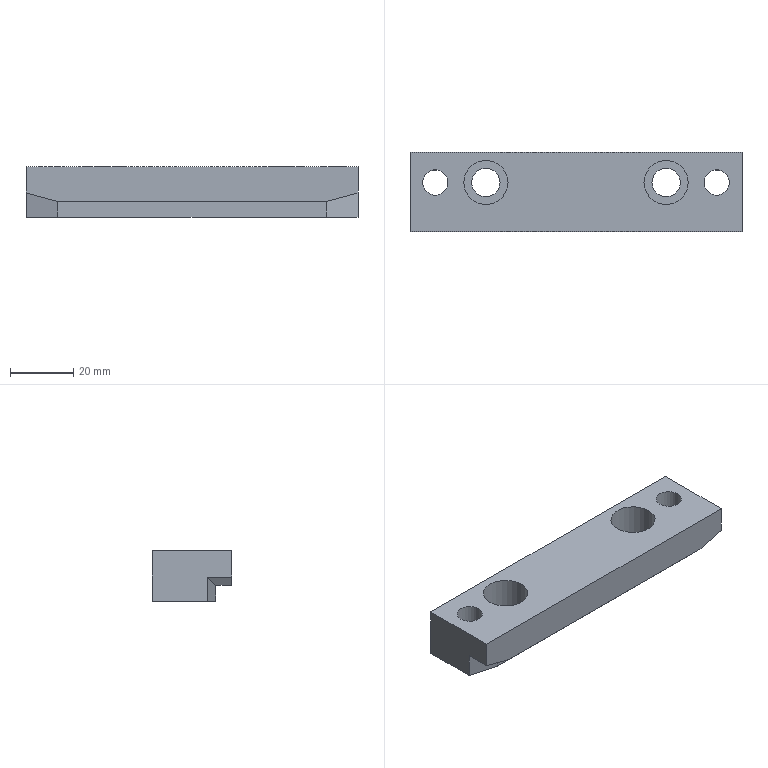Part | STEP file | 1 solid | 20 faces | box 105 x 25 x 16 mm | volume 33608 mm3 | plane 14 | cylinder 6 | commonest cylinder face diameters 8 x2 9 x2 14 x2
STEP:
#1=CARTESIAN_POINT('',(20.,96.9,3.));
#2=VERTEX_POINT('',#1);
#3=CARTESIAN_POINT('',(30.,99.58,5.679));
#4=VERTEX_POINT('',#3);
#5=CARTESIAN_POINT('',(35.23,100.981,7.081));
#6=DIRECTION('',(0.9351,0.2506,0.2506));
#7=VECTOR('',#6,1.);
#8=LINE('',#5,#7);
#9=EDGE_CURVE('',#2,#4,#8,.T.);
#10=ORIENTED_EDGE('',*,*,#9,.T.);
#11=CARTESIAN_POINT('',(30.,91.9,5.679));
#12=VERTEX_POINT('',#11);
#13=CARTESIAN_POINT('',(30.,89.4,5.679));
#14=DIRECTION('',(0.,-1.,0.));
#15=VECTOR('',#14,1.);
#16=LINE('',#13,#15);
#17=EDGE_CURVE('',#4,#12,#16,.T.);
#18=ORIENTED_EDGE('',*,*,#17,.T.);
#19=CARTESIAN_POINT('',(20.,91.9,3.));
#20=VERTEX_POINT('',#19);
#21=CARTESIAN_POINT('',(27.33,91.9,4.964));
#22=DIRECTION('',(-0.9659,0.,-0.2588));
#23=VECTOR('',#22,1.);
#24=LINE('',#21,#23);
#25=EDGE_CURVE('',#12,#20,#24,.T.);
#26=ORIENTED_EDGE('',*,*,#25,.T.);
#27=CARTESIAN_POINT('',(20.,97.08,3.));
#28=DIRECTION('',(0.,1.,0.));
#29=VECTOR('',#28,1.);
#30=LINE('',#27,#29);
#31=EDGE_CURVE('',#20,#2,#30,.T.);
#32=ORIENTED_EDGE('',*,*,#31,.T.);
#33=EDGE_LOOP('',(#10,#18,#26,#32));
#34=FACE_OUTER_BOUND('',#33,.T.);
#35=CARTESIAN_POINT('',(30.,119.4,5.679));
#36=DIRECTION('',(0.2588,0.,-0.9659));
#37=DIRECTION('',(0.9659,0.,0.2588));
#38=AXIS2_PLACEMENT_3D('',#35,#36,#37);
#39=PLANE('',#38);
#40=ADVANCED_FACE('',(#34),#39,.T.);
#41=CARTESIAN_POINT('',(-65.,96.9,3.));
#42=VERTEX_POINT('',#41);
#43=CARTESIAN_POINT('',(-125.,96.9,3.));
#44=DIRECTION('',(-1.,0.,0.));
#45=VECTOR('',#44,1.);
#46=LINE('',#43,#45);
#47=EDGE_CURVE('',#2,#42,#46,.T.);
#48=ORIENTED_EDGE('',*,*,#47,.F.);
#49=ORIENTED_EDGE('',*,*,#31,.F.);
#50=CARTESIAN_POINT('',(-65.,91.9,3.));
#51=VERTEX_POINT('',#50);
#52=CARTESIAN_POINT('',(-35.,91.9,3.));
#53=DIRECTION('',(1.,0.,0.));
#54=VECTOR('',#53,1.);
#55=LINE('',#52,#54);
#56=EDGE_CURVE('',#51,#20,#55,.T.);
#57=ORIENTED_EDGE('',*,*,#56,.F.);
#58=CARTESIAN_POINT('',(-65.,97.08,3.));
#59=DIRECTION('',(0.,1.,0.));
#60=VECTOR('',#59,1.);
#61=LINE('',#58,#60);
#62=EDGE_CURVE('',#51,#42,#61,.T.);
#63=ORIENTED_EDGE('',*,*,#62,.T.);
#64=EDGE_LOOP('',(#48,#49,#57,#63));
#65=FACE_OUTER_BOUND('',#64,.T.);
#66=CARTESIAN_POINT('',(-46.,107.4,3.));
#67=DIRECTION('',(0.,0.,1.));
#68=DIRECTION('',(-1.,0.,0.));
#69=AXIS2_PLACEMENT_3D('',#66,#67,#68);
#70=PLANE('',#69);
#71=ADVANCED_FACE('',(#65),#70,.F.);
#72=CARTESIAN_POINT('',(-75.,99.58,5.679));
#73=VERTEX_POINT('',#72);
#74=CARTESIAN_POINT('',(-80.23,100.981,7.081));
#75=DIRECTION('',(-0.9351,0.2506,0.2506));
#76=VECTOR('',#75,1.);
#77=LINE('',#74,#76);
#78=EDGE_CURVE('',#42,#73,#77,.T.);
#79=ORIENTED_EDGE('',*,*,#78,.F.);
#80=ORIENTED_EDGE('',*,*,#62,.F.);
#81=CARTESIAN_POINT('',(-75.,91.9,5.679));
#82=VERTEX_POINT('',#81);
#83=CARTESIAN_POINT('',(-72.33,91.9,4.964));
#84=DIRECTION('',(0.9659,0.,-0.2588));
#85=VECTOR('',#84,1.);
#86=LINE('',#83,#85);
#87=EDGE_CURVE('',#82,#51,#86,.T.);
#88=ORIENTED_EDGE('',*,*,#87,.F.);
#89=CARTESIAN_POINT('',(-75.,89.4,5.679));
#90=DIRECTION('',(0.,-1.,0.));
#91=VECTOR('',#90,1.);
#92=LINE('',#89,#91);
#93=EDGE_CURVE('',#73,#82,#92,.T.);
#94=ORIENTED_EDGE('',*,*,#93,.F.);
#95=EDGE_LOOP('',(#79,#80,#88,#94));
#96=FACE_OUTER_BOUND('',#95,.T.);
#97=CARTESIAN_POINT('',(-75.,119.4,5.679));
#98=DIRECTION('',(-0.2588,0.,-0.9659));
#99=DIRECTION('',(-0.9659,0.,0.2588));
#100=AXIS2_PLACEMENT_3D('',#97,#98,#99);
#101=PLANE('',#100);
#102=ADVANCED_FACE('',(#96),#101,.T.);
#103=CARTESIAN_POINT('',(-64.998,96.9,-2.));
#104=VERTEX_POINT('',#103);
#105=CARTESIAN_POINT('',(-64.998,96.9,14.));
#106=DIRECTION('',(0.,0.,1.));
#107=VECTOR('',#106,1.);
#108=LINE('',#105,#107);
#109=EDGE_CURVE('',#104,#42,#108,.T.);
#110=ORIENTED_EDGE('',*,*,#109,.T.);
#111=ORIENTED_EDGE('',*,*,#78,.T.);
#112=CARTESIAN_POINT('',(-75.,99.58,-2.));
#113=VERTEX_POINT('',#112);
#114=CARTESIAN_POINT('',(-75.,99.58,-2.));
#115=DIRECTION('',(0.,0.,1.));
#116=VECTOR('',#115,1.);
#117=LINE('',#114,#116);
#118=EDGE_CURVE('',#113,#73,#117,.T.);
#119=ORIENTED_EDGE('',*,*,#118,.F.);
#120=CARTESIAN_POINT('',(-67.317,97.521,-2.));
#121=DIRECTION('',(0.9659,-0.2588,0.));
#122=VECTOR('',#121,1.);
#123=LINE('',#120,#122);
#124=EDGE_CURVE('',#113,#104,#123,.T.);
#125=ORIENTED_EDGE('',*,*,#124,.T.);
#126=EDGE_LOOP('',(#110,#111,#119,#125));
#127=FACE_OUTER_BOUND('',#126,.T.);
#128=CARTESIAN_POINT('',(-65.,96.9,14.));
#129=DIRECTION('',(-0.2588,-0.9659,0.));
#130=DIRECTION('',(0.9659,-0.2588,0.));
#131=AXIS2_PLACEMENT_3D('',#128,#129,#130);
#132=PLANE('',#131);
#133=ADVANCED_FACE('',(#127),#132,.T.);
#134=ORIENTED_EDGE('',*,*,#47,.T.);
#135=ORIENTED_EDGE('',*,*,#109,.F.);
#136=CARTESIAN_POINT('',(19.998,96.9,-2.));
#137=VERTEX_POINT('',#136);
#138=CARTESIAN_POINT('',(-46.,96.9,-2.));
#139=DIRECTION('',(1.,0.,0.));
#140=VECTOR('',#139,1.);
#141=LINE('',#138,#140);
#142=EDGE_CURVE('',#104,#137,#141,.T.);
#143=ORIENTED_EDGE('',*,*,#142,.T.);
#144=CARTESIAN_POINT('',(19.998,96.9,14.));
#145=DIRECTION('',(0.,0.,1.));
#146=VECTOR('',#145,1.);
#147=LINE('',#144,#146);
#148=EDGE_CURVE('',#137,#2,#147,.T.);
#149=ORIENTED_EDGE('',*,*,#148,.T.);
#150=EDGE_LOOP('',(#134,#135,#143,#149));
#151=FACE_OUTER_BOUND('',#150,.T.);
#152=CARTESIAN_POINT('',(-125.,96.9,14.));
#153=DIRECTION('',(0.,-1.,0.));
#154=DIRECTION('',(0.,0.,-1.));
#155=AXIS2_PLACEMENT_3D('',#152,#153,#154);
#156=PLANE('',#155);
#157=ADVANCED_FACE('',(#151),#156,.T.);
#158=ORIENTED_EDGE('',*,*,#148,.F.);
#159=CARTESIAN_POINT('',(30.,99.58,-2.));
#160=VERTEX_POINT('',#159);
#161=CARTESIAN_POINT('',(22.317,97.521,-2.));
#162=DIRECTION('',(-0.9659,-0.2588,0.));
#163=VECTOR('',#162,1.);
#164=LINE('',#161,#163);
#165=EDGE_CURVE('',#160,#137,#164,.T.);
#166=ORIENTED_EDGE('',*,*,#165,.F.);
#167=CARTESIAN_POINT('',(30.,99.58,-2.));
#168=DIRECTION('',(0.,0.,1.));
#169=VECTOR('',#168,1.);
#170=LINE('',#167,#169);
#171=EDGE_CURVE('',#160,#4,#170,.T.);
#172=ORIENTED_EDGE('',*,*,#171,.T.);
#173=ORIENTED_EDGE('',*,*,#9,.F.);
#174=EDGE_LOOP('',(#158,#166,#172,#173));
#175=FACE_OUTER_BOUND('',#174,.T.);
#176=CARTESIAN_POINT('',(20.,96.9,14.));
#177=DIRECTION('',(0.2588,-0.9659,0.));
#178=DIRECTION('',(-0.9659,-0.2588,0.));
#179=AXIS2_PLACEMENT_3D('',#176,#177,#178);
#180=PLANE('',#179);
#181=ADVANCED_FACE('',(#175),#180,.T.);
#182=ORIENTED_EDGE('',*,*,#171,.F.);
#183=CARTESIAN_POINT('',(30.,116.9,-2.));
#184=VERTEX_POINT('',#183);
#185=CARTESIAN_POINT('',(30.,119.4,-2.));
#186=DIRECTION('',(0.,-1.,0.));
#187=VECTOR('',#186,1.);
#188=LINE('',#185,#187);
#189=EDGE_CURVE('',#184,#160,#188,.T.);
#190=ORIENTED_EDGE('',*,*,#189,.F.);
#191=CARTESIAN_POINT('',(30.,116.9,14.));
#192=VERTEX_POINT('',#191);
#193=CARTESIAN_POINT('',(30.,116.9,-2.));
#194=DIRECTION('',(0.,0.,1.));
#195=VECTOR('',#194,1.);
#196=LINE('',#193,#195);
#197=EDGE_CURVE('',#184,#192,#196,.T.);
#198=ORIENTED_EDGE('',*,*,#197,.T.);
#199=CARTESIAN_POINT('',(30.,91.9,14.));
#200=VERTEX_POINT('',#199);
#201=CARTESIAN_POINT('',(30.,119.4,14.));
#202=DIRECTION('',(0.,-1.,0.));
#203=VECTOR('',#202,1.);
#204=LINE('',#201,#203);
#205=EDGE_CURVE('',#192,#200,#204,.T.);
#206=ORIENTED_EDGE('',*,*,#205,.T.);
#207=CARTESIAN_POINT('',(30.,91.9,-2.));
#208=DIRECTION('',(0.,0.,1.));
#209=VECTOR('',#208,1.);
#210=LINE('',#207,#209);
#211=EDGE_CURVE('',#12,#200,#210,.T.);
#212=ORIENTED_EDGE('',*,*,#211,.F.);
#213=ORIENTED_EDGE('',*,*,#17,.F.);
#214=EDGE_LOOP('',(#182,#190,#198,#206,#212,#213));
#215=FACE_OUTER_BOUND('',#214,.T.);
#216=CARTESIAN_POINT('',(30.,119.4,-2.));
#217=DIRECTION('',(1.,0.,0.));
#218=DIRECTION('',(0.,0.,1.));
#219=AXIS2_PLACEMENT_3D('',#216,#217,#218);
#220=PLANE('',#219);
#221=ADVANCED_FACE('',(#215),#220,.T.);
#222=CARTESIAN_POINT('',(-75.,91.9,14.));
#223=VERTEX_POINT('',#222);
#224=CARTESIAN_POINT('',(-35.,91.9,14.));
#225=DIRECTION('',(1.,0.,0.));
#226=VECTOR('',#225,1.);
#227=LINE('',#224,#226);
#228=EDGE_CURVE('',#223,#200,#227,.T.);
#229=ORIENTED_EDGE('',*,*,#228,.F.);
#230=CARTESIAN_POINT('',(-75.,91.9,-2.));
#231=DIRECTION('',(0.,0.,1.));
#232=VECTOR('',#231,1.);
#233=LINE('',#230,#232);
#234=EDGE_CURVE('',#82,#223,#233,.T.);
#235=ORIENTED_EDGE('',*,*,#234,.F.);
#236=ORIENTED_EDGE('',*,*,#87,.T.);
#237=ORIENTED_EDGE('',*,*,#56,.T.);
#238=ORIENTED_EDGE('',*,*,#25,.F.);
#239=ORIENTED_EDGE('',*,*,#211,.T.);
#240=EDGE_LOOP('',(#229,#235,#236,#237,#238,#239));
#241=FACE_OUTER_BOUND('',#240,.T.);
#242=CARTESIAN_POINT('',(-35.,91.9,-2.));
#243=DIRECTION('',(0.,-1.,0.));
#244=DIRECTION('',(0.,0.,-1.));
#245=AXIS2_PLACEMENT_3D('',#242,#243,#244);
#246=PLANE('',#245);
#247=ADVANCED_FACE('',(#241),#246,.T.);
#248=ORIENTED_EDGE('',*,*,#118,.T.);
#249=ORIENTED_EDGE('',*,*,#93,.T.);
#250=ORIENTED_EDGE('',*,*,#234,.T.);
#251=CARTESIAN_POINT('',(-75.,116.9,14.));
#252=VERTEX_POINT('',#251);
#253=CARTESIAN_POINT('',(-75.,119.4,14.));
#254=DIRECTION('',(0.,-1.,0.));
#255=VECTOR('',#254,1.);
#256=LINE('',#253,#255);
#257=EDGE_CURVE('',#252,#223,#256,.T.);
#258=ORIENTED_EDGE('',*,*,#257,.F.);
#259=CARTESIAN_POINT('',(-75.,116.9,-2.));
#260=VERTEX_POINT('',#259);
#261=CARTESIAN_POINT('',(-75.,116.9,-2.));
#262=DIRECTION('',(0.,0.,1.));
#263=VECTOR('',#262,1.);
#264=LINE('',#261,#263);
#265=EDGE_CURVE('',#260,#252,#264,.T.);
#266=ORIENTED_EDGE('',*,*,#265,.F.);
#267=CARTESIAN_POINT('',(-75.,119.4,-2.));
#268=DIRECTION('',(0.,-1.,0.));
#269=VECTOR('',#268,1.);
#270=LINE('',#267,#269);
#271=EDGE_CURVE('',#260,#113,#270,.T.);
#272=ORIENTED_EDGE('',*,*,#271,.T.);
#273=EDGE_LOOP('',(#248,#249,#250,#258,#266,#272));
#274=FACE_OUTER_BOUND('',#273,.T.);
#275=CARTESIAN_POINT('',(-75.,119.4,-2.));
#276=DIRECTION('',(-1.,0.,0.));
#277=DIRECTION('',(0.,0.,1.));
#278=AXIS2_PLACEMENT_3D('',#275,#276,#277);
#279=PLANE('',#278);
#280=ADVANCED_FACE('',(#274),#279,.T.);
#281=CARTESIAN_POINT('',(-46.,116.9,-2.));
#282=DIRECTION('',(-1.,0.,0.));
#283=VECTOR('',#282,1.);
#284=LINE('',#281,#283);
#285=EDGE_CURVE('',#184,#260,#284,.T.);
#286=ORIENTED_EDGE('',*,*,#285,.T.);
#287=ORIENTED_EDGE('',*,*,#265,.T.);
#288=CARTESIAN_POINT('',(-46.,116.9,14.));
#289=DIRECTION('',(-1.,0.,0.));
#290=VECTOR('',#289,1.);
#291=LINE('',#288,#290);
#292=EDGE_CURVE('',#192,#252,#291,.T.);
#293=ORIENTED_EDGE('',*,*,#292,.F.);
#294=ORIENTED_EDGE('',*,*,#197,.F.);
#295=EDGE_LOOP('',(#286,#287,#293,#294));
#296=FACE_OUTER_BOUND('',#295,.T.);
#297=CARTESIAN_POINT('',(-135.,116.9,-2.));
#298=DIRECTION('',(0.,1.,0.));
#299=DIRECTION('',(0.,0.,1.));
#300=AXIS2_PLACEMENT_3D('',#297,#298,#299);
#301=PLANE('',#300);
#302=ADVANCED_FACE('',(#296),#301,.T.);
#303=CARTESIAN_POINT('',(-58.,107.4,14.));
#304=VERTEX_POINT('',#303);
#305=CARTESIAN_POINT('',(-51.,107.4,14.));
#306=DIRECTION('',(0.,0.,1.));
#307=DIRECTION('',(-1.,0.,0.));
#308=AXIS2_PLACEMENT_3D('',#305,#306,#307);
#309=CIRCLE('',#308,7.);
#310=EDGE_CURVE('',#304,#304,#309,.T.);
#311=ORIENTED_EDGE('',*,*,#310,.F.);
#312=EDGE_LOOP('',(#311));
#313=FACE_BOUND('',#312,.T.);
#314=CARTESIAN_POINT('',(-71.,107.4,14.));
#315=VERTEX_POINT('',#314);
#316=CARTESIAN_POINT('',(-67.,107.4,14.));
#317=DIRECTION('',(0.,0.,1.));
#318=DIRECTION('',(-1.,0.,0.));
#319=AXIS2_PLACEMENT_3D('',#316,#317,#318);
#320=CIRCLE('',#319,4.);
#321=EDGE_CURVE('',#315,#315,#320,.T.);
#322=ORIENTED_EDGE('',*,*,#321,.F.);
#323=EDGE_LOOP('',(#322));
#324=FACE_BOUND('',#323,.T.);
#325=CARTESIAN_POINT('',(13.,107.4,14.));
#326=VERTEX_POINT('',#325);
#327=CARTESIAN_POINT('',(6.,107.4,14.));
#328=DIRECTION('',(0.,0.,-1.));
#329=DIRECTION('',(1.,0.,0.));
#330=AXIS2_PLACEMENT_3D('',#327,#328,#329);
#331=CIRCLE('',#330,7.);
#332=EDGE_CURVE('',#326,#326,#331,.T.);
#333=ORIENTED_EDGE('',*,*,#332,.T.);
#334=EDGE_LOOP('',(#333));
#335=FACE_BOUND('',#334,.T.);
#336=CARTESIAN_POINT('',(26.,107.4,14.));
#337=VERTEX_POINT('',#336);
#338=CARTESIAN_POINT('',(22.,107.4,14.));
#339=DIRECTION('',(0.,0.,-1.));
#340=DIRECTION('',(1.,0.,0.));
#341=AXIS2_PLACEMENT_3D('',#338,#339,#340);
#342=CIRCLE('',#341,4.);
#343=EDGE_CURVE('',#337,#337,#342,.T.);
#344=ORIENTED_EDGE('',*,*,#343,.T.);
#345=EDGE_LOOP('',(#344));
#346=FACE_BOUND('',#345,.T.);
#347=ORIENTED_EDGE('',*,*,#292,.T.);
#348=ORIENTED_EDGE('',*,*,#257,.T.);
#349=ORIENTED_EDGE('',*,*,#228,.T.);
#350=ORIENTED_EDGE('',*,*,#205,.F.);
#351=EDGE_LOOP('',(#347,#348,#349,#350));
#352=FACE_BOUND('',#351,.T.);
#353=CARTESIAN_POINT('',(-46.,107.4,14.));
#354=DIRECTION('',(0.,0.,1.));
#355=DIRECTION('',(-1.,0.,0.));
#356=AXIS2_PLACEMENT_3D('',#353,#354,#355);
#357=PLANE('',#356);
#358=ADVANCED_FACE('',(#313,#324,#335,#346,#352),#357,.T.);
#359=CARTESIAN_POINT('',(-55.5,107.4,-2.));
#360=VERTEX_POINT('',#359);
#361=CARTESIAN_POINT('',(-51.,107.4,-2.));
#362=DIRECTION('',(0.,0.,-1.));
#363=DIRECTION('',(-1.,0.,0.));
#364=AXIS2_PLACEMENT_3D('',#361,#362,#363);
#365=CIRCLE('',#364,4.5);
#366=EDGE_CURVE('',#360,#360,#365,.T.);
#367=ORIENTED_EDGE('',*,*,#366,.F.);
#368=EDGE_LOOP('',(#367));
#369=FACE_BOUND('',#368,.T.);
#370=CARTESIAN_POINT('',(-71.,107.4,-2.));
#371=VERTEX_POINT('',#370);
#372=CARTESIAN_POINT('',(-67.,107.4,-2.));
#373=DIRECTION('',(0.,0.,-1.));
#374=DIRECTION('',(-1.,0.,0.));
#375=AXIS2_PLACEMENT_3D('',#372,#373,#374);
#376=CIRCLE('',#375,4.);
#377=EDGE_CURVE('',#371,#371,#376,.T.);
#378=ORIENTED_EDGE('',*,*,#377,.F.);
#379=EDGE_LOOP('',(#378));
#380=FACE_BOUND('',#379,.T.);
#381=CARTESIAN_POINT('',(10.5,107.4,-2.));
#382=VERTEX_POINT('',#381);
#383=CARTESIAN_POINT('',(6.,107.4,-2.));
#384=DIRECTION('',(0.,0.,1.));
#385=DIRECTION('',(1.,0.,0.));
#386=AXIS2_PLACEMENT_3D('',#383,#384,#385);
#387=CIRCLE('',#386,4.5);
#388=EDGE_CURVE('',#382,#382,#387,.T.);
#389=ORIENTED_EDGE('',*,*,#388,.T.);
#390=EDGE_LOOP('',(#389));
#391=FACE_BOUND('',#390,.T.);
#392=CARTESIAN_POINT('',(26.,107.4,-2.));
#393=VERTEX_POINT('',#392);
#394=CARTESIAN_POINT('',(22.,107.4,-2.));
#395=DIRECTION('',(0.,0.,1.));
#396=DIRECTION('',(1.,0.,0.));
#397=AXIS2_PLACEMENT_3D('',#394,#395,#396);
#398=CIRCLE('',#397,4.);
#399=EDGE_CURVE('',#393,#393,#398,.T.);
#400=ORIENTED_EDGE('',*,*,#399,.T.);
#401=EDGE_LOOP('',(#400));
#402=FACE_BOUND('',#401,.T.);
#403=ORIENTED_EDGE('',*,*,#285,.F.);
#404=ORIENTED_EDGE('',*,*,#189,.T.);
#405=ORIENTED_EDGE('',*,*,#165,.T.);
#406=ORIENTED_EDGE('',*,*,#142,.F.);
#407=ORIENTED_EDGE('',*,*,#124,.F.);
#408=ORIENTED_EDGE('',*,*,#271,.F.);
#409=EDGE_LOOP('',(#403,#404,#405,#406,#407,#408));
#410=FACE_BOUND('',#409,.T.);
#411=CARTESIAN_POINT('',(-46.,107.4,-2.));
#412=DIRECTION('',(0.,0.,1.));
#413=DIRECTION('',(-1.,0.,0.));
#414=AXIS2_PLACEMENT_3D('',#411,#412,#413);
#415=PLANE('',#414);
#416=ADVANCED_FACE('',(#369,#380,#391,#402,#410),#415,.F.);
#417=ORIENTED_EDGE('',*,*,#343,.F.);
#418=EDGE_LOOP('',(#417));
#419=FACE_BOUND('',#418,.T.);
#420=ORIENTED_EDGE('',*,*,#399,.F.);
#421=EDGE_LOOP('',(#420));
#422=FACE_BOUND('',#421,.T.);
#423=CARTESIAN_POINT('',(22.,107.4,-2.));
#424=DIRECTION('',(0.,0.,1.));
#425=DIRECTION('',(1.,0.,0.));
#426=AXIS2_PLACEMENT_3D('',#423,#424,#425);
#427=CYLINDRICAL_SURFACE('',#426,4.);
#428=ADVANCED_FACE('',(#419,#422),#427,.F.);
#429=CARTESIAN_POINT('',(1.5,107.4,4.));
#430=VERTEX_POINT('',#429);
#431=CARTESIAN_POINT('',(6.,107.4,4.));
#432=DIRECTION('',(0.,0.,-1.));
#433=DIRECTION('',(-1.,0.,0.));
#434=AXIS2_PLACEMENT_3D('',#431,#432,#433);
#435=CIRCLE('',#434,4.5);
#436=EDGE_CURVE('',#430,#430,#435,.T.);
#437=ORIENTED_EDGE('',*,*,#436,.F.);
#438=EDGE_LOOP('',(#437));
#439=FACE_BOUND('',#438,.T.);
#440=ORIENTED_EDGE('',*,*,#388,.F.);
#441=EDGE_LOOP('',(#440));
#442=FACE_BOUND('',#441,.T.);
#443=CARTESIAN_POINT('',(6.,107.4,-2.));
#444=DIRECTION('',(0.,0.,1.));
#445=DIRECTION('',(1.,0.,0.));
#446=AXIS2_PLACEMENT_3D('',#443,#444,#445);
#447=CYLINDRICAL_SURFACE('',#446,4.5);
#448=ADVANCED_FACE('',(#439,#442),#447,.F.);
#449=ORIENTED_EDGE('',*,*,#436,.T.);
#450=EDGE_LOOP('',(#449));
#451=FACE_BOUND('',#450,.T.);
#452=CARTESIAN_POINT('',(13.,107.4,4.));
#453=VERTEX_POINT('',#452);
#454=CARTESIAN_POINT('',(6.,107.4,4.));
#455=DIRECTION('',(0.,0.,-1.));
#456=DIRECTION('',(1.,0.,0.));
#457=AXIS2_PLACEMENT_3D('',#454,#455,#456);
#458=CIRCLE('',#457,7.);
#459=EDGE_CURVE('',#453,#453,#458,.T.);
#460=ORIENTED_EDGE('',*,*,#459,.F.);
#461=EDGE_LOOP('',(#460));
#462=FACE_BOUND('',#461,.T.);
#463=CARTESIAN_POINT('',(6.,107.4,4.));
#464=DIRECTION('',(0.,0.,-1.));
#465=DIRECTION('',(-1.,0.,0.));
#466=AXIS2_PLACEMENT_3D('',#463,#464,#465);
#467=PLANE('',#466);
#468=ADVANCED_FACE('',(#451,#462),#467,.F.);
#469=ORIENTED_EDGE('',*,*,#332,.F.);
#470=EDGE_LOOP('',(#469));
#471=FACE_BOUND('',#470,.T.);
#472=ORIENTED_EDGE('',*,*,#459,.T.);
#473=EDGE_LOOP('',(#472));
#474=FACE_BOUND('',#473,.T.);
#475=CARTESIAN_POINT('',(6.,107.4,4.));
#476=DIRECTION('',(0.,0.,1.));
#477=DIRECTION('',(1.,0.,0.));
#478=AXIS2_PLACEMENT_3D('',#475,#476,#477);
#479=CYLINDRICAL_SURFACE('',#478,7.);
#480=ADVANCED_FACE('',(#471,#474),#479,.F.);
#481=ORIENTED_EDGE('',*,*,#321,.T.);
#482=EDGE_LOOP('',(#481));
#483=FACE_BOUND('',#482,.T.);
#484=ORIENTED_EDGE('',*,*,#377,.T.);
#485=EDGE_LOOP('',(#484));
#486=FACE_BOUND('',#485,.T.);
#487=CARTESIAN_POINT('',(-67.,107.4,-2.));
#488=DIRECTION('',(0.,0.,1.));
#489=DIRECTION('',(-1.,0.,0.));
#490=AXIS2_PLACEMENT_3D('',#487,#488,#489);
#491=CYLINDRICAL_SURFACE('',#490,4.);
#492=ADVANCED_FACE('',(#483,#486),#491,.F.);
#493=CARTESIAN_POINT('',(-46.5,107.4,4.));
#494=VERTEX_POINT('',#493);
#495=CARTESIAN_POINT('',(-51.,107.4,4.));
#496=DIRECTION('',(0.,0.,1.));
#497=DIRECTION('',(1.,0.,0.));
#498=AXIS2_PLACEMENT_3D('',#495,#496,#497);
#499=CIRCLE('',#498,4.5);
#500=EDGE_CURVE('',#494,#494,#499,.T.);
#501=ORIENTED_EDGE('',*,*,#500,.T.);
#502=EDGE_LOOP('',(#501));
#503=FACE_BOUND('',#502,.T.);
#504=ORIENTED_EDGE('',*,*,#366,.T.);
#505=EDGE_LOOP('',(#504));
#506=FACE_BOUND('',#505,.T.);
#507=CARTESIAN_POINT('',(-51.,107.4,-2.));
#508=DIRECTION('',(0.,0.,1.));
#509=DIRECTION('',(-1.,0.,0.));
#510=AXIS2_PLACEMENT_3D('',#507,#508,#509);
#511=CYLINDRICAL_SURFACE('',#510,4.5);
#512=ADVANCED_FACE('',(#503,#506),#511,.F.);
#513=ORIENTED_EDGE('',*,*,#500,.F.);
#514=EDGE_LOOP('',(#513));
#515=FACE_BOUND('',#514,.T.);
#516=CARTESIAN_POINT('',(-58.,107.4,4.));
#517=VERTEX_POINT('',#516);
#518=CARTESIAN_POINT('',(-51.,107.4,4.));
#519=DIRECTION('',(0.,0.,1.));
#520=DIRECTION('',(-1.,0.,0.));
#521=AXIS2_PLACEMENT_3D('',#518,#519,#520);
#522=CIRCLE('',#521,7.);
#523=EDGE_CURVE('',#517,#517,#522,.T.);
#524=ORIENTED_EDGE('',*,*,#523,.T.);
#525=EDGE_LOOP('',(#524));
#526=FACE_BOUND('',#525,.T.);
#527=CARTESIAN_POINT('',(-51.,107.4,4.));
#528=DIRECTION('',(0.,0.,-1.));
#529=DIRECTION('',(1.,0.,0.));
#530=AXIS2_PLACEMENT_3D('',#527,#528,#529);
#531=PLANE('',#530);
#532=ADVANCED_FACE('',(#515,#526),#531,.F.);
#533=ORIENTED_EDGE('',*,*,#310,.T.);
#534=EDGE_LOOP('',(#533));
#535=FACE_BOUND('',#534,.T.);
#536=ORIENTED_EDGE('',*,*,#523,.F.);
#537=EDGE_LOOP('',(#536));
#538=FACE_BOUND('',#537,.T.);
#539=CARTESIAN_POINT('',(-51.,107.4,4.));
#540=DIRECTION('',(0.,0.,1.));
#541=DIRECTION('',(-1.,0.,0.));
#542=AXIS2_PLACEMENT_3D('',#539,#540,#541);
#543=CYLINDRICAL_SURFACE('',#542,7.);
#544=ADVANCED_FACE('',(#535,#538),#543,.F.);
#545=CLOSED_SHELL('',(#40,#71,#102,#133,#157,#181,#221,#247,#280,#302,#358,#416,#428,#448,#468,#480,#492,#512,#532,#544));
#546=MANIFOLD_SOLID_BREP('',#545);
#547=(LENGTH_UNIT()NAMED_UNIT(*)SI_UNIT(.MILLI.,.METRE.));
#548=UNCERTAINTY_MEASURE_WITH_UNIT(LENGTH_MEASURE(0.002713),#547,'','');
#549=(NAMED_UNIT(*)PLANE_ANGLE_UNIT()SI_UNIT($,.RADIAN.));
#550=PLANE_ANGLE_MEASURE_WITH_UNIT(PLANE_ANGLE_MEASURE(0.01745),#549);
#551=DIMENSIONAL_EXPONENTS(0.,0.,0.,0.,0.,0.,0.);
#552=(CONVERSION_BASED_UNIT('DEGREE',#550)NAMED_UNIT(#551)PLANE_ANGLE_UNIT());
#553=(NAMED_UNIT(*)SI_UNIT($,.STERADIAN.)SOLID_ANGLE_UNIT());
#554=(GEOMETRIC_REPRESENTATION_CONTEXT(3)GLOBAL_UNCERTAINTY_ASSIGNED_CONTEXT((#548))GLOBAL_UNIT_ASSIGNED_CONTEXT((#547,#552,#553))REPRESENTATION_CONTEXT('',''));
#555=ADVANCED_BREP_SHAPE_REPRESENTATION('',(#546),#554);